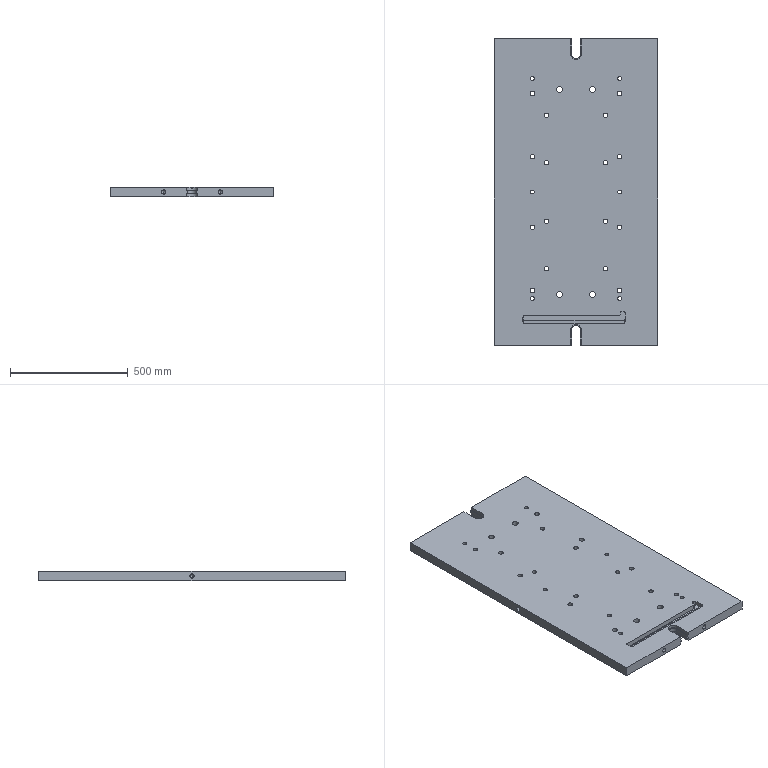Part | STEP file | 4-20.sldasm-Part-328 | 1 solid | 183 faces | box 692.15 x 1300 x 41.275 mm | volume 36129684 mm3 | cylinder 106 | plane 57 | cone 20 | commonest cylinder face diameters 19.05 x28 19.842 x16 30.162 x16 16.667 x12 25.4 x12 33.496 x8